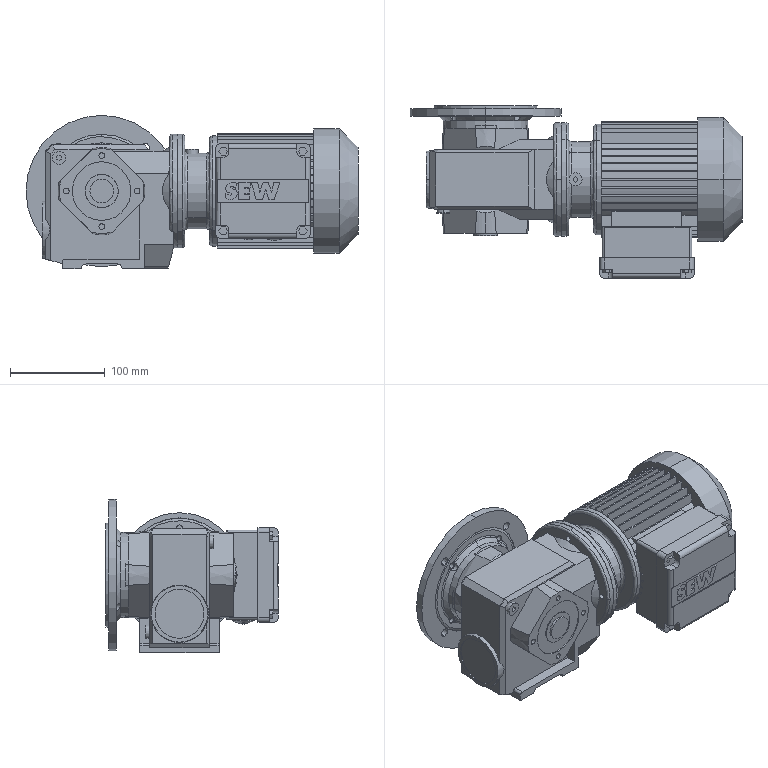Part | SolidWorks | 14 solids | 657 faces | box 351 x 182.5 x 162 mm | volume 4012734 mm3 | plane 453 | cylinder 154 | cone 30 | spline 20 | commonest cylinder face diameters 6 x30 10 x14 6.6 x8 7 x8 9 x8 9.9 x6